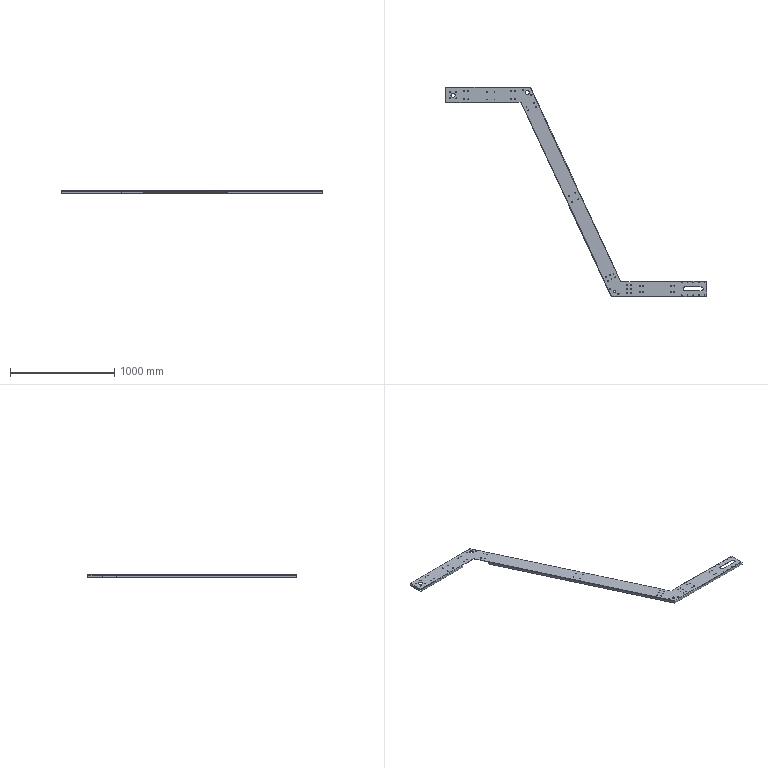Part | STEP file | Produce dryer-Conveyor side plate 1 | 1 solid | 221 faces | box 2506 x 2006 x 25 mm | volume 2012083 mm3 | cylinder 141 | plane 76 | spline 4 | commonest cylinder face diameters 9 x80 5 x20 11 x16 2 x8 8 x8 40 x7